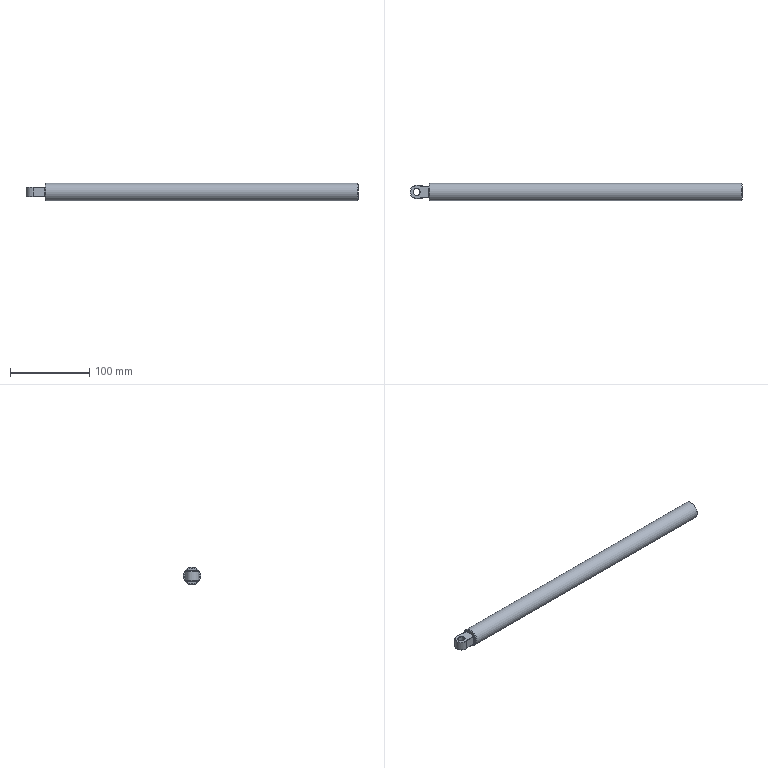Part | STEP file | GAS SHOCK A01X | 1 solid | 30 faces | box 419 x 22 x 22 mm | volume 110141 mm3 | cylinder 12 | plane 7 | torus 7 | spline 4 | commonest cylinder face diameters 1 x8 8.2 x1 12 x1 17 x1 22 x1